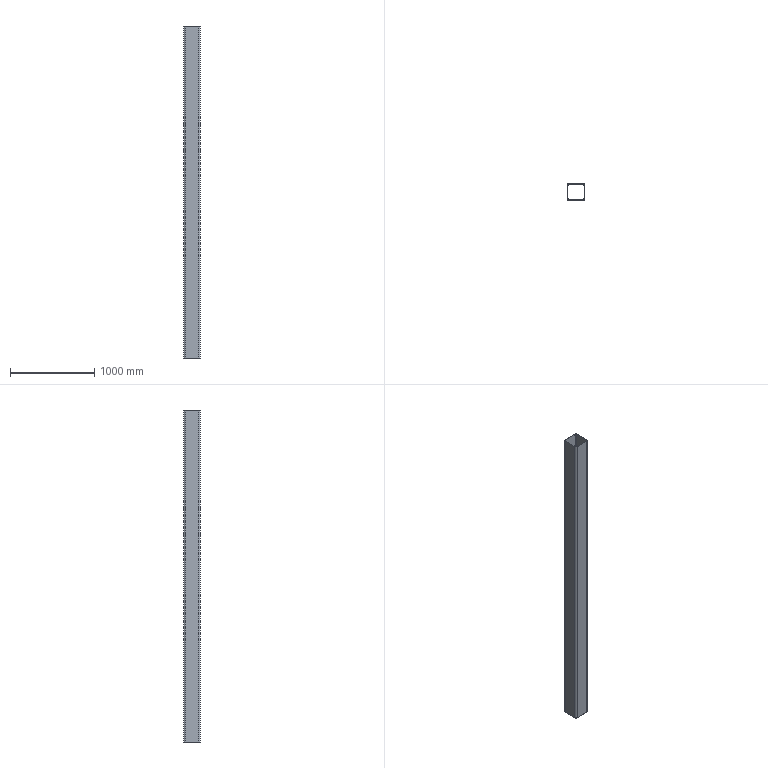Part | SolidWorks | features Extrusion 1 | 1 solid | 18 faces | box 200 x 200 x 3930 mm | volume 14736630 mm3 | plane 10 | cylinder 8 | commonest cylinder face diameters 30 x4 40 x4
STEP:
#1=CARTESIAN_POINT('',(-100.,-80.,3930.));
#2=VERTEX_POINT('',#1);
#3=CARTESIAN_POINT('',(-80.,-100.,3930.));
#4=VERTEX_POINT('',#3);
#5=CARTESIAN_POINT('',(-80.,-80.,3930.));
#6=DIRECTION('',(0.,0.,1.));
#7=DIRECTION('',(1.,0.,0.));
#8=AXIS2_PLACEMENT_3D('',#5,#6,#7);
#9=CIRCLE('',#8,20.);
#10=EDGE_CURVE('',#2,#4,#9,.T.);
#11=ORIENTED_EDGE('',*,*,#10,.T.);
#12=CARTESIAN_POINT('',(80.,-100.,3930.));
#13=VERTEX_POINT('',#12);
#14=CARTESIAN_POINT('',(-80.,-100.,3930.));
#15=DIRECTION('',(1.,0.,0.));
#16=VECTOR('',#15,1000.);
#17=LINE('',#14,#16);
#18=EDGE_CURVE('',#4,#13,#17,.T.);
#19=ORIENTED_EDGE('',*,*,#18,.T.);
#20=CARTESIAN_POINT('',(100.,-80.,3930.));
#21=VERTEX_POINT('',#20);
#22=CARTESIAN_POINT('',(80.,-80.,3930.));
#23=DIRECTION('',(0.,0.,1.));
#24=DIRECTION('',(1.,0.,0.));
#25=AXIS2_PLACEMENT_3D('',#22,#23,#24);
#26=CIRCLE('',#25,20.);
#27=EDGE_CURVE('',#13,#21,#26,.T.);
#28=ORIENTED_EDGE('',*,*,#27,.T.);
#29=CARTESIAN_POINT('',(100.,80.,3930.));
#30=VERTEX_POINT('',#29);
#31=CARTESIAN_POINT('',(100.,80.,3930.));
#32=DIRECTION('',(0.,1.,0.));
#33=VECTOR('',#32,1000.);
#34=LINE('',#31,#33);
#35=EDGE_CURVE('',#21,#30,#34,.T.);
#36=ORIENTED_EDGE('',*,*,#35,.T.);
#37=CARTESIAN_POINT('',(80.,100.,3930.));
#38=VERTEX_POINT('',#37);
#39=CARTESIAN_POINT('',(80.,80.,3930.));
#40=DIRECTION('',(0.,0.,1.));
#41=DIRECTION('',(-1.,0.,0.));
#42=AXIS2_PLACEMENT_3D('',#39,#40,#41);
#43=CIRCLE('',#42,20.);
#44=EDGE_CURVE('',#30,#38,#43,.T.);
#45=ORIENTED_EDGE('',*,*,#44,.T.);
#46=CARTESIAN_POINT('',(-80.,100.,3930.));
#47=VERTEX_POINT('',#46);
#48=CARTESIAN_POINT('',(-80.,100.,3930.));
#49=DIRECTION('',(-1.,0.,0.));
#50=VECTOR('',#49,1000.);
#51=LINE('',#48,#50);
#52=EDGE_CURVE('',#38,#47,#51,.T.);
#53=ORIENTED_EDGE('',*,*,#52,.T.);
#54=CARTESIAN_POINT('',(-100.,80.,3930.));
#55=VERTEX_POINT('',#54);
#56=CARTESIAN_POINT('',(-80.,80.,3930.));
#57=DIRECTION('',(0.,0.,1.));
#58=DIRECTION('',(1.,0.,0.));
#59=AXIS2_PLACEMENT_3D('',#56,#57,#58);
#60=CIRCLE('',#59,20.);
#61=EDGE_CURVE('',#47,#55,#60,.T.);
#62=ORIENTED_EDGE('',*,*,#61,.T.);
#63=CARTESIAN_POINT('',(-100.,80.,3930.));
#64=DIRECTION('',(0.,-1.,0.));
#65=VECTOR('',#64,1000.);
#66=LINE('',#63,#65);
#67=EDGE_CURVE('',#55,#2,#66,.T.);
#68=ORIENTED_EDGE('',*,*,#67,.T.);
#69=EDGE_LOOP('',(#11,#19,#28,#36,#45,#53,#62,#68));
#70=FACE_OUTER_BOUND('',#69,.T.);
#71=CARTESIAN_POINT('',(-95.,80.,3930.));
#72=VERTEX_POINT('',#71);
#73=CARTESIAN_POINT('',(-95.,-80.,3930.));
#74=VERTEX_POINT('',#73);
#75=CARTESIAN_POINT('',(-95.,80.,3930.));
#76=DIRECTION('',(0.,-1.,0.));
#77=VECTOR('',#76,1000.);
#78=LINE('',#75,#77);
#79=EDGE_CURVE('',#72,#74,#78,.T.);
#80=ORIENTED_EDGE('',*,*,#79,.F.);
#81=CARTESIAN_POINT('',(-80.,95.,3930.));
#82=VERTEX_POINT('',#81);
#83=CARTESIAN_POINT('',(-80.,80.,3930.));
#84=DIRECTION('',(0.,0.,1.));
#85=DIRECTION('',(1.,0.,0.));
#86=AXIS2_PLACEMENT_3D('',#83,#84,#85);
#87=CIRCLE('',#86,15.);
#88=EDGE_CURVE('',#82,#72,#87,.T.);
#89=ORIENTED_EDGE('',*,*,#88,.F.);
#90=CARTESIAN_POINT('',(80.,95.,3930.));
#91=VERTEX_POINT('',#90);
#92=CARTESIAN_POINT('',(-80.,95.,3930.));
#93=DIRECTION('',(-1.,0.,0.));
#94=VECTOR('',#93,1000.);
#95=LINE('',#92,#94);
#96=EDGE_CURVE('',#91,#82,#95,.T.);
#97=ORIENTED_EDGE('',*,*,#96,.F.);
#98=CARTESIAN_POINT('',(95.,80.,3930.));
#99=VERTEX_POINT('',#98);
#100=CARTESIAN_POINT('',(80.,80.,3930.));
#101=DIRECTION('',(0.,0.,1.));
#102=DIRECTION('',(-1.,0.,0.));
#103=AXIS2_PLACEMENT_3D('',#100,#101,#102);
#104=CIRCLE('',#103,15.);
#105=EDGE_CURVE('',#99,#91,#104,.T.);
#106=ORIENTED_EDGE('',*,*,#105,.F.);
#107=CARTESIAN_POINT('',(95.,-80.,3930.));
#108=VERTEX_POINT('',#107);
#109=CARTESIAN_POINT('',(95.,80.,3930.));
#110=DIRECTION('',(0.,1.,0.));
#111=VECTOR('',#110,1000.);
#112=LINE('',#109,#111);
#113=EDGE_CURVE('',#108,#99,#112,.T.);
#114=ORIENTED_EDGE('',*,*,#113,.F.);
#115=CARTESIAN_POINT('',(80.,-95.,3930.));
#116=VERTEX_POINT('',#115);
#117=CARTESIAN_POINT('',(80.,-80.,3930.));
#118=DIRECTION('',(0.,0.,1.));
#119=DIRECTION('',(1.,0.,0.));
#120=AXIS2_PLACEMENT_3D('',#117,#118,#119);
#121=CIRCLE('',#120,15.);
#122=EDGE_CURVE('',#116,#108,#121,.T.);
#123=ORIENTED_EDGE('',*,*,#122,.F.);
#124=CARTESIAN_POINT('',(-80.,-95.,3930.));
#125=VERTEX_POINT('',#124);
#126=CARTESIAN_POINT('',(-80.,-95.,3930.));
#127=DIRECTION('',(1.,0.,0.));
#128=VECTOR('',#127,1000.);
#129=LINE('',#126,#128);
#130=EDGE_CURVE('',#125,#116,#129,.T.);
#131=ORIENTED_EDGE('',*,*,#130,.F.);
#132=CARTESIAN_POINT('',(-80.,-80.,3930.));
#133=DIRECTION('',(0.,0.,1.));
#134=DIRECTION('',(1.,0.,0.));
#135=AXIS2_PLACEMENT_3D('',#132,#133,#134);
#136=CIRCLE('',#135,15.);
#137=EDGE_CURVE('',#74,#125,#136,.T.);
#138=ORIENTED_EDGE('',*,*,#137,.F.);
#139=EDGE_LOOP('',(#80,#89,#97,#106,#114,#123,#131,#138));
#140=FACE_BOUND('',#139,.T.);
#141=CARTESIAN_POINT('',(-80.,-80.,3930.));
#142=DIRECTION('',(0.,0.,1.));
#143=DIRECTION('',(1.,0.,0.));
#144=AXIS2_PLACEMENT_3D('',#141,#142,#143);
#145=PLANE('',#144);
#146=ADVANCED_FACE('',(#70,#140),#145,.T.);
#147=CARTESIAN_POINT('',(-100.,-80.,0.));
#148=VERTEX_POINT('',#147);
#149=CARTESIAN_POINT('',(-80.,-100.,0.));
#150=VERTEX_POINT('',#149);
#151=CARTESIAN_POINT('',(-80.,-80.,0.));
#152=DIRECTION('',(0.,0.,1.));
#153=DIRECTION('',(1.,0.,0.));
#154=AXIS2_PLACEMENT_3D('',#151,#152,#153);
#155=CIRCLE('',#154,20.);
#156=EDGE_CURVE('',#148,#150,#155,.T.);
#157=ORIENTED_EDGE('',*,*,#156,.F.);
#158=CARTESIAN_POINT('',(-100.,80.,0.));
#159=VERTEX_POINT('',#158);
#160=CARTESIAN_POINT('',(-100.,80.,0.));
#161=DIRECTION('',(0.,-1.,0.));
#162=VECTOR('',#161,1000.);
#163=LINE('',#160,#162);
#164=EDGE_CURVE('',#159,#148,#163,.T.);
#165=ORIENTED_EDGE('',*,*,#164,.F.);
#166=CARTESIAN_POINT('',(-80.,100.,0.));
#167=VERTEX_POINT('',#166);
#168=CARTESIAN_POINT('',(-80.,80.,0.));
#169=DIRECTION('',(0.,0.,1.));
#170=DIRECTION('',(1.,0.,0.));
#171=AXIS2_PLACEMENT_3D('',#168,#169,#170);
#172=CIRCLE('',#171,20.);
#173=EDGE_CURVE('',#167,#159,#172,.T.);
#174=ORIENTED_EDGE('',*,*,#173,.F.);
#175=CARTESIAN_POINT('',(80.,100.,0.));
#176=VERTEX_POINT('',#175);
#177=CARTESIAN_POINT('',(-80.,100.,0.));
#178=DIRECTION('',(-1.,0.,0.));
#179=VECTOR('',#178,1000.);
#180=LINE('',#177,#179);
#181=EDGE_CURVE('',#176,#167,#180,.T.);
#182=ORIENTED_EDGE('',*,*,#181,.F.);
#183=CARTESIAN_POINT('',(100.,80.,0.));
#184=VERTEX_POINT('',#183);
#185=CARTESIAN_POINT('',(80.,80.,0.));
#186=DIRECTION('',(0.,0.,1.));
#187=DIRECTION('',(-1.,0.,0.));
#188=AXIS2_PLACEMENT_3D('',#185,#186,#187);
#189=CIRCLE('',#188,20.);
#190=EDGE_CURVE('',#184,#176,#189,.T.);
#191=ORIENTED_EDGE('',*,*,#190,.F.);
#192=CARTESIAN_POINT('',(100.,-80.,0.));
#193=VERTEX_POINT('',#192);
#194=CARTESIAN_POINT('',(100.,80.,0.));
#195=DIRECTION('',(0.,1.,0.));
#196=VECTOR('',#195,1000.);
#197=LINE('',#194,#196);
#198=EDGE_CURVE('',#193,#184,#197,.T.);
#199=ORIENTED_EDGE('',*,*,#198,.F.);
#200=CARTESIAN_POINT('',(80.,-100.,0.));
#201=VERTEX_POINT('',#200);
#202=CARTESIAN_POINT('',(80.,-80.,0.));
#203=DIRECTION('',(0.,0.,1.));
#204=DIRECTION('',(1.,0.,0.));
#205=AXIS2_PLACEMENT_3D('',#202,#203,#204);
#206=CIRCLE('',#205,20.);
#207=EDGE_CURVE('',#201,#193,#206,.T.);
#208=ORIENTED_EDGE('',*,*,#207,.F.);
#209=CARTESIAN_POINT('',(-80.,-100.,0.));
#210=DIRECTION('',(1.,0.,0.));
#211=VECTOR('',#210,1000.);
#212=LINE('',#209,#211);
#213=EDGE_CURVE('',#150,#201,#212,.T.);
#214=ORIENTED_EDGE('',*,*,#213,.F.);
#215=EDGE_LOOP('',(#157,#165,#174,#182,#191,#199,#208,#214));
#216=FACE_OUTER_BOUND('',#215,.T.);
#217=CARTESIAN_POINT('',(-80.,95.,0.));
#218=VERTEX_POINT('',#217);
#219=CARTESIAN_POINT('',(-95.,80.,0.));
#220=VERTEX_POINT('',#219);
#221=CARTESIAN_POINT('',(-80.,80.,0.));
#222=DIRECTION('',(0.,0.,1.));
#223=DIRECTION('',(1.,0.,0.));
#224=AXIS2_PLACEMENT_3D('',#221,#222,#223);
#225=CIRCLE('',#224,15.);
#226=EDGE_CURVE('',#218,#220,#225,.T.);
#227=ORIENTED_EDGE('',*,*,#226,.T.);
#228=CARTESIAN_POINT('',(-95.,-80.,0.));
#229=VERTEX_POINT('',#228);
#230=CARTESIAN_POINT('',(-95.,80.,0.));
#231=DIRECTION('',(0.,-1.,0.));
#232=VECTOR('',#231,1000.);
#233=LINE('',#230,#232);
#234=EDGE_CURVE('',#220,#229,#233,.T.);
#235=ORIENTED_EDGE('',*,*,#234,.T.);
#236=CARTESIAN_POINT('',(-80.,-95.,0.));
#237=VERTEX_POINT('',#236);
#238=CARTESIAN_POINT('',(-80.,-80.,0.));
#239=DIRECTION('',(0.,0.,1.));
#240=DIRECTION('',(1.,0.,0.));
#241=AXIS2_PLACEMENT_3D('',#238,#239,#240);
#242=CIRCLE('',#241,15.);
#243=EDGE_CURVE('',#229,#237,#242,.T.);
#244=ORIENTED_EDGE('',*,*,#243,.T.);
#245=CARTESIAN_POINT('',(80.,-95.,0.));
#246=VERTEX_POINT('',#245);
#247=CARTESIAN_POINT('',(-80.,-95.,0.));
#248=DIRECTION('',(1.,0.,0.));
#249=VECTOR('',#248,1000.);
#250=LINE('',#247,#249);
#251=EDGE_CURVE('',#237,#246,#250,.T.);
#252=ORIENTED_EDGE('',*,*,#251,.T.);
#253=CARTESIAN_POINT('',(95.,-80.,0.));
#254=VERTEX_POINT('',#253);
#255=CARTESIAN_POINT('',(80.,-80.,0.));
#256=DIRECTION('',(0.,0.,1.));
#257=DIRECTION('',(1.,0.,0.));
#258=AXIS2_PLACEMENT_3D('',#255,#256,#257);
#259=CIRCLE('',#258,15.);
#260=EDGE_CURVE('',#246,#254,#259,.T.);
#261=ORIENTED_EDGE('',*,*,#260,.T.);
#262=CARTESIAN_POINT('',(95.,80.,0.));
#263=VERTEX_POINT('',#262);
#264=CARTESIAN_POINT('',(95.,80.,0.));
#265=DIRECTION('',(0.,1.,0.));
#266=VECTOR('',#265,1000.);
#267=LINE('',#264,#266);
#268=EDGE_CURVE('',#254,#263,#267,.T.);
#269=ORIENTED_EDGE('',*,*,#268,.T.);
#270=CARTESIAN_POINT('',(80.,95.,0.));
#271=VERTEX_POINT('',#270);
#272=CARTESIAN_POINT('',(80.,80.,0.));
#273=DIRECTION('',(0.,0.,1.));
#274=DIRECTION('',(-1.,0.,0.));
#275=AXIS2_PLACEMENT_3D('',#272,#273,#274);
#276=CIRCLE('',#275,15.);
#277=EDGE_CURVE('',#263,#271,#276,.T.);
#278=ORIENTED_EDGE('',*,*,#277,.T.);
#279=CARTESIAN_POINT('',(-80.,95.,0.));
#280=DIRECTION('',(-1.,0.,0.));
#281=VECTOR('',#280,1000.);
#282=LINE('',#279,#281);
#283=EDGE_CURVE('',#271,#218,#282,.T.);
#284=ORIENTED_EDGE('',*,*,#283,.T.);
#285=EDGE_LOOP('',(#227,#235,#244,#252,#261,#269,#278,#284));
#286=FACE_BOUND('',#285,.T.);
#287=CARTESIAN_POINT('',(-80.,-80.,0.));
#288=DIRECTION('',(0.,0.,1.));
#289=DIRECTION('',(1.,0.,0.));
#290=AXIS2_PLACEMENT_3D('',#287,#288,#289);
#291=PLANE('',#290);
#292=ADVANCED_FACE('',(#216,#286),#291,.F.);
#293=ORIENTED_EDGE('',*,*,#156,.T.);
#294=CARTESIAN_POINT('',(-80.,-100.,3930.));
#295=DIRECTION('',(0.,0.,-1.));
#296=VECTOR('',#295,1000.);
#297=LINE('',#294,#296);
#298=EDGE_CURVE('',#4,#150,#297,.T.);
#299=ORIENTED_EDGE('',*,*,#298,.F.);
#300=ORIENTED_EDGE('',*,*,#10,.F.);
#301=CARTESIAN_POINT('',(-100.,-80.,3930.));
#302=DIRECTION('',(0.,0.,-1.));
#303=VECTOR('',#302,1000.);
#304=LINE('',#301,#303);
#305=EDGE_CURVE('',#2,#148,#304,.T.);
#306=ORIENTED_EDGE('',*,*,#305,.T.);
#307=EDGE_LOOP('',(#293,#299,#300,#306));
#308=FACE_OUTER_BOUND('',#307,.T.);
#309=CARTESIAN_POINT('',(-80.,-80.,3930.));
#310=DIRECTION('',(0.,0.,-1.));
#311=DIRECTION('',(-1.,0.,0.));
#312=AXIS2_PLACEMENT_3D('',#309,#310,#311);
#313=CYLINDRICAL_SURFACE('',#312,20.);
#314=ADVANCED_FACE('',(#308),#313,.T.);
#315=ORIENTED_EDGE('',*,*,#213,.T.);
#316=CARTESIAN_POINT('',(80.,-100.,3930.));
#317=DIRECTION('',(0.,0.,-1.));
#318=VECTOR('',#317,1000.);
#319=LINE('',#316,#318);
#320=EDGE_CURVE('',#13,#201,#319,.T.);
#321=ORIENTED_EDGE('',*,*,#320,.F.);
#322=ORIENTED_EDGE('',*,*,#18,.F.);
#323=ORIENTED_EDGE('',*,*,#298,.T.);
#324=EDGE_LOOP('',(#315,#321,#322,#323));
#325=FACE_OUTER_BOUND('',#324,.T.);
#326=CARTESIAN_POINT('',(-80.,-100.,3930.));
#327=DIRECTION('',(0.,1.,0.));
#328=DIRECTION('',(0.,0.,1.));
#329=AXIS2_PLACEMENT_3D('',#326,#327,#328);
#330=PLANE('',#329);
#331=ADVANCED_FACE('',(#325),#330,.F.);
#332=ORIENTED_EDGE('',*,*,#207,.T.);
#333=CARTESIAN_POINT('',(100.,-80.,3930.));
#334=DIRECTION('',(0.,0.,-1.));
#335=VECTOR('',#334,1000.);
#336=LINE('',#333,#335);
#337=EDGE_CURVE('',#21,#193,#336,.T.);
#338=ORIENTED_EDGE('',*,*,#337,.F.);
#339=ORIENTED_EDGE('',*,*,#27,.F.);
#340=ORIENTED_EDGE('',*,*,#320,.T.);
#341=EDGE_LOOP('',(#332,#338,#339,#340));
#342=FACE_OUTER_BOUND('',#341,.T.);
#343=CARTESIAN_POINT('',(80.,-80.,3930.));
#344=DIRECTION('',(0.,0.,-1.));
#345=DIRECTION('',(-1.,0.,0.));
#346=AXIS2_PLACEMENT_3D('',#343,#344,#345);
#347=CYLINDRICAL_SURFACE('',#346,20.);
#348=ADVANCED_FACE('',(#342),#347,.T.);
#349=ORIENTED_EDGE('',*,*,#198,.T.);
#350=CARTESIAN_POINT('',(100.,80.,3930.));
#351=DIRECTION('',(0.,0.,-1.));
#352=VECTOR('',#351,1000.);
#353=LINE('',#350,#352);
#354=EDGE_CURVE('',#30,#184,#353,.T.);
#355=ORIENTED_EDGE('',*,*,#354,.F.);
#356=ORIENTED_EDGE('',*,*,#35,.F.);
#357=ORIENTED_EDGE('',*,*,#337,.T.);
#358=EDGE_LOOP('',(#349,#355,#356,#357));
#359=FACE_OUTER_BOUND('',#358,.T.);
#360=CARTESIAN_POINT('',(100.,80.,3930.));
#361=DIRECTION('',(-1.,0.,0.));
#362=DIRECTION('',(0.,-1.,0.));
#363=AXIS2_PLACEMENT_3D('',#360,#361,#362);
#364=PLANE('',#363);
#365=ADVANCED_FACE('',(#359),#364,.F.);
#366=ORIENTED_EDGE('',*,*,#190,.T.);
#367=CARTESIAN_POINT('',(80.,100.,3930.));
#368=DIRECTION('',(0.,0.,-1.));
#369=VECTOR('',#368,1000.);
#370=LINE('',#367,#369);
#371=EDGE_CURVE('',#38,#176,#370,.T.);
#372=ORIENTED_EDGE('',*,*,#371,.F.);
#373=ORIENTED_EDGE('',*,*,#44,.F.);
#374=ORIENTED_EDGE('',*,*,#354,.T.);
#375=EDGE_LOOP('',(#366,#372,#373,#374));
#376=FACE_OUTER_BOUND('',#375,.T.);
#377=CARTESIAN_POINT('',(80.,80.,3930.));
#378=DIRECTION('',(0.,0.,-1.));
#379=DIRECTION('',(-1.,0.,0.));
#380=AXIS2_PLACEMENT_3D('',#377,#378,#379);
#381=CYLINDRICAL_SURFACE('',#380,20.);
#382=ADVANCED_FACE('',(#376),#381,.T.);
#383=ORIENTED_EDGE('',*,*,#181,.T.);
#384=CARTESIAN_POINT('',(-80.,100.,3930.));
#385=DIRECTION('',(0.,0.,-1.));
#386=VECTOR('',#385,1000.);
#387=LINE('',#384,#386);
#388=EDGE_CURVE('',#47,#167,#387,.T.);
#389=ORIENTED_EDGE('',*,*,#388,.F.);
#390=ORIENTED_EDGE('',*,*,#52,.F.);
#391=ORIENTED_EDGE('',*,*,#371,.T.);
#392=EDGE_LOOP('',(#383,#389,#390,#391));
#393=FACE_OUTER_BOUND('',#392,.T.);
#394=CARTESIAN_POINT('',(-80.,100.,3930.));
#395=DIRECTION('',(0.,-1.,0.));
#396=DIRECTION('',(0.,0.,-1.));
#397=AXIS2_PLACEMENT_3D('',#394,#395,#396);
#398=PLANE('',#397);
#399=ADVANCED_FACE('',(#393),#398,.F.);
#400=ORIENTED_EDGE('',*,*,#173,.T.);
#401=CARTESIAN_POINT('',(-100.,80.,3930.));
#402=DIRECTION('',(0.,0.,-1.));
#403=VECTOR('',#402,1000.);
#404=LINE('',#401,#403);
#405=EDGE_CURVE('',#55,#159,#404,.T.);
#406=ORIENTED_EDGE('',*,*,#405,.F.);
#407=ORIENTED_EDGE('',*,*,#61,.F.);
#408=ORIENTED_EDGE('',*,*,#388,.T.);
#409=EDGE_LOOP('',(#400,#406,#407,#408));
#410=FACE_OUTER_BOUND('',#409,.T.);
#411=CARTESIAN_POINT('',(-80.,80.,3930.));
#412=DIRECTION('',(0.,0.,-1.));
#413=DIRECTION('',(-1.,0.,0.));
#414=AXIS2_PLACEMENT_3D('',#411,#412,#413);
#415=CYLINDRICAL_SURFACE('',#414,20.);
#416=ADVANCED_FACE('',(#410),#415,.T.);
#417=ORIENTED_EDGE('',*,*,#164,.T.);
#418=ORIENTED_EDGE('',*,*,#305,.F.);
#419=ORIENTED_EDGE('',*,*,#67,.F.);
#420=ORIENTED_EDGE('',*,*,#405,.T.);
#421=EDGE_LOOP('',(#417,#418,#419,#420));
#422=FACE_OUTER_BOUND('',#421,.T.);
#423=CARTESIAN_POINT('',(-100.,80.,3930.));
#424=DIRECTION('',(1.,0.,0.));
#425=DIRECTION('',(0.,1.,0.));
#426=AXIS2_PLACEMENT_3D('',#423,#424,#425);
#427=PLANE('',#426);
#428=ADVANCED_FACE('',(#422),#427,.F.);
#429=ORIENTED_EDGE('',*,*,#226,.F.);
#430=CARTESIAN_POINT('',(-80.,95.,3930.));
#431=DIRECTION('',(0.,0.,-1.));
#432=VECTOR('',#431,1000.);
#433=LINE('',#430,#432);
#434=EDGE_CURVE('',#82,#218,#433,.T.);
#435=ORIENTED_EDGE('',*,*,#434,.F.);
#436=ORIENTED_EDGE('',*,*,#88,.T.);
#437=CARTESIAN_POINT('',(-95.,80.,3930.));
#438=DIRECTION('',(0.,0.,-1.));
#439=VECTOR('',#438,1000.);
#440=LINE('',#437,#439);
#441=EDGE_CURVE('',#72,#220,#440,.T.);
#442=ORIENTED_EDGE('',*,*,#441,.T.);
#443=EDGE_LOOP('',(#429,#435,#436,#442));
#444=FACE_OUTER_BOUND('',#443,.T.);
#445=CARTESIAN_POINT('',(-80.,80.,3930.));
#446=DIRECTION('',(0.,0.,-1.));
#447=DIRECTION('',(-1.,0.,0.));
#448=AXIS2_PLACEMENT_3D('',#445,#446,#447);
#449=CYLINDRICAL_SURFACE('',#448,15.);
#450=ADVANCED_FACE('',(#444),#449,.F.);
#451=ORIENTED_EDGE('',*,*,#234,.F.);
#452=ORIENTED_EDGE('',*,*,#441,.F.);
#453=ORIENTED_EDGE('',*,*,#79,.T.);
#454=CARTESIAN_POINT('',(-95.,-80.,3930.));
#455=DIRECTION('',(0.,0.,-1.));
#456=VECTOR('',#455,1000.);
#457=LINE('',#454,#456);
#458=EDGE_CURVE('',#74,#229,#457,.T.);
#459=ORIENTED_EDGE('',*,*,#458,.T.);
#460=EDGE_LOOP('',(#451,#452,#453,#459));
#461=FACE_OUTER_BOUND('',#460,.T.);
#462=CARTESIAN_POINT('',(-95.,80.,3930.));
#463=DIRECTION('',(1.,0.,0.));
#464=DIRECTION('',(0.,1.,0.));
#465=AXIS2_PLACEMENT_3D('',#462,#463,#464);
#466=PLANE('',#465);
#467=ADVANCED_FACE('',(#461),#466,.T.);
#468=ORIENTED_EDGE('',*,*,#243,.F.);
#469=ORIENTED_EDGE('',*,*,#458,.F.);
#470=ORIENTED_EDGE('',*,*,#137,.T.);
#471=CARTESIAN_POINT('',(-80.,-95.,3930.));
#472=DIRECTION('',(0.,0.,-1.));
#473=VECTOR('',#472,1000.);
#474=LINE('',#471,#473);
#475=EDGE_CURVE('',#125,#237,#474,.T.);
#476=ORIENTED_EDGE('',*,*,#475,.T.);
#477=EDGE_LOOP('',(#468,#469,#470,#476));
#478=FACE_OUTER_BOUND('',#477,.T.);
#479=CARTESIAN_POINT('',(-80.,-80.,3930.));
#480=DIRECTION('',(0.,0.,-1.));
#481=DIRECTION('',(-1.,0.,0.));
#482=AXIS2_PLACEMENT_3D('',#479,#480,#481);
#483=CYLINDRICAL_SURFACE('',#482,15.);
#484=ADVANCED_FACE('',(#478),#483,.F.);
#485=ORIENTED_EDGE('',*,*,#251,.F.);
#486=ORIENTED_EDGE('',*,*,#475,.F.);
#487=ORIENTED_EDGE('',*,*,#130,.T.);
#488=CARTESIAN_POINT('',(80.,-95.,3930.));
#489=DIRECTION('',(0.,0.,-1.));
#490=VECTOR('',#489,1000.);
#491=LINE('',#488,#490);
#492=EDGE_CURVE('',#116,#246,#491,.T.);
#493=ORIENTED_EDGE('',*,*,#492,.T.);
#494=EDGE_LOOP('',(#485,#486,#487,#493));
#495=FACE_OUTER_BOUND('',#494,.T.);
#496=CARTESIAN_POINT('',(-80.,-95.,3930.));
#497=DIRECTION('',(0.,1.,0.));
#498=DIRECTION('',(0.,0.,1.));
#499=AXIS2_PLACEMENT_3D('',#496,#497,#498);
#500=PLANE('',#499);
#501=ADVANCED_FACE('',(#495),#500,.T.);
#502=ORIENTED_EDGE('',*,*,#260,.F.);
#503=ORIENTED_EDGE('',*,*,#492,.F.);
#504=ORIENTED_EDGE('',*,*,#122,.T.);
#505=CARTESIAN_POINT('',(95.,-80.,3930.));
#506=DIRECTION('',(0.,0.,-1.));
#507=VECTOR('',#506,1000.);
#508=LINE('',#505,#507);
#509=EDGE_CURVE('',#108,#254,#508,.T.);
#510=ORIENTED_EDGE('',*,*,#509,.T.);
#511=EDGE_LOOP('',(#502,#503,#504,#510));
#512=FACE_OUTER_BOUND('',#511,.T.);
#513=CARTESIAN_POINT('',(80.,-80.,3930.));
#514=DIRECTION('',(0.,0.,-1.));
#515=DIRECTION('',(-1.,0.,0.));
#516=AXIS2_PLACEMENT_3D('',#513,#514,#515);
#517=CYLINDRICAL_SURFACE('',#516,15.);
#518=ADVANCED_FACE('',(#512),#517,.F.);
#519=ORIENTED_EDGE('',*,*,#268,.F.);
#520=ORIENTED_EDGE('',*,*,#509,.F.);
#521=ORIENTED_EDGE('',*,*,#113,.T.);
#522=CARTESIAN_POINT('',(95.,80.,3930.));
#523=DIRECTION('',(0.,0.,-1.));
#524=VECTOR('',#523,1000.);
#525=LINE('',#522,#524);
#526=EDGE_CURVE('',#99,#263,#525,.T.);
#527=ORIENTED_EDGE('',*,*,#526,.T.);
#528=EDGE_LOOP('',(#519,#520,#521,#527));
#529=FACE_OUTER_BOUND('',#528,.T.);
#530=CARTESIAN_POINT('',(95.,80.,3930.));
#531=DIRECTION('',(-1.,0.,0.));
#532=DIRECTION('',(0.,-1.,0.));
#533=AXIS2_PLACEMENT_3D('',#530,#531,#532);
#534=PLANE('',#533);
#535=ADVANCED_FACE('',(#529),#534,.T.);
#536=ORIENTED_EDGE('',*,*,#277,.F.);
#537=ORIENTED_EDGE('',*,*,#526,.F.);
#538=ORIENTED_EDGE('',*,*,#105,.T.);
#539=CARTESIAN_POINT('',(80.,95.,3930.));
#540=DIRECTION('',(0.,0.,-1.));
#541=VECTOR('',#540,1000.);
#542=LINE('',#539,#541);
#543=EDGE_CURVE('',#91,#271,#542,.T.);
#544=ORIENTED_EDGE('',*,*,#543,.T.);
#545=EDGE_LOOP('',(#536,#537,#538,#544));
#546=FACE_OUTER_BOUND('',#545,.T.);
#547=CARTESIAN_POINT('',(80.,80.,3930.));
#548=DIRECTION('',(0.,0.,-1.));
#549=DIRECTION('',(-1.,0.,0.));
#550=AXIS2_PLACEMENT_3D('',#547,#548,#549);
#551=CYLINDRICAL_SURFACE('',#550,15.);
#552=ADVANCED_FACE('',(#546),#551,.F.);
#553=ORIENTED_EDGE('',*,*,#283,.F.);
#554=ORIENTED_EDGE('',*,*,#543,.F.);
#555=ORIENTED_EDGE('',*,*,#96,.T.);
#556=ORIENTED_EDGE('',*,*,#434,.T.);
#557=EDGE_LOOP('',(#553,#554,#555,#556));
#558=FACE_OUTER_BOUND('',#557,.T.);
#559=CARTESIAN_POINT('',(-80.,95.,3930.));
#560=DIRECTION('',(0.,-1.,0.));
#561=DIRECTION('',(0.,0.,-1.));
#562=AXIS2_PLACEMENT_3D('',#559,#560,#561);
#563=PLANE('',#562);
#564=ADVANCED_FACE('',(#558),#563,.T.);
#565=CLOSED_SHELL('',(#146,#292,#314,#331,#348,#365,#382,#399,#416,#428,#450,#467,#484,#501,#518,#535,#552,#564));
#566=MANIFOLD_SOLID_BREP('',#565);
#567=CARTESIAN_POINT('',(0.,0.,0.));
#568=DIRECTION('',(0.,0.,1.));
#569=DIRECTION('',(1.,0.,0.));
#570=AXIS2_PLACEMENT_3D('',#567,#568,#569);
#571=(LENGTH_UNIT()NAMED_UNIT(*)SI_UNIT(.MILLI.,.METRE.));
#572=UNCERTAINTY_MEASURE_WITH_UNIT(LENGTH_MEASURE(0.00001),#571,'','');
#573=(NAMED_UNIT(*)PLANE_ANGLE_UNIT()SI_UNIT($,.RADIAN.));
#574=(NAMED_UNIT(*)SI_UNIT($,.STERADIAN.)SOLID_ANGLE_UNIT());
#575=(GEOMETRIC_REPRESENTATION_CONTEXT(3)GLOBAL_UNCERTAINTY_ASSIGNED_CONTEXT((#572))GLOBAL_UNIT_ASSIGNED_CONTEXT((#571,#573,#574))REPRESENTATION_CONTEXT('',''));
#576=ADVANCED_BREP_SHAPE_REPRESENTATION('',(#566,#570),#575);